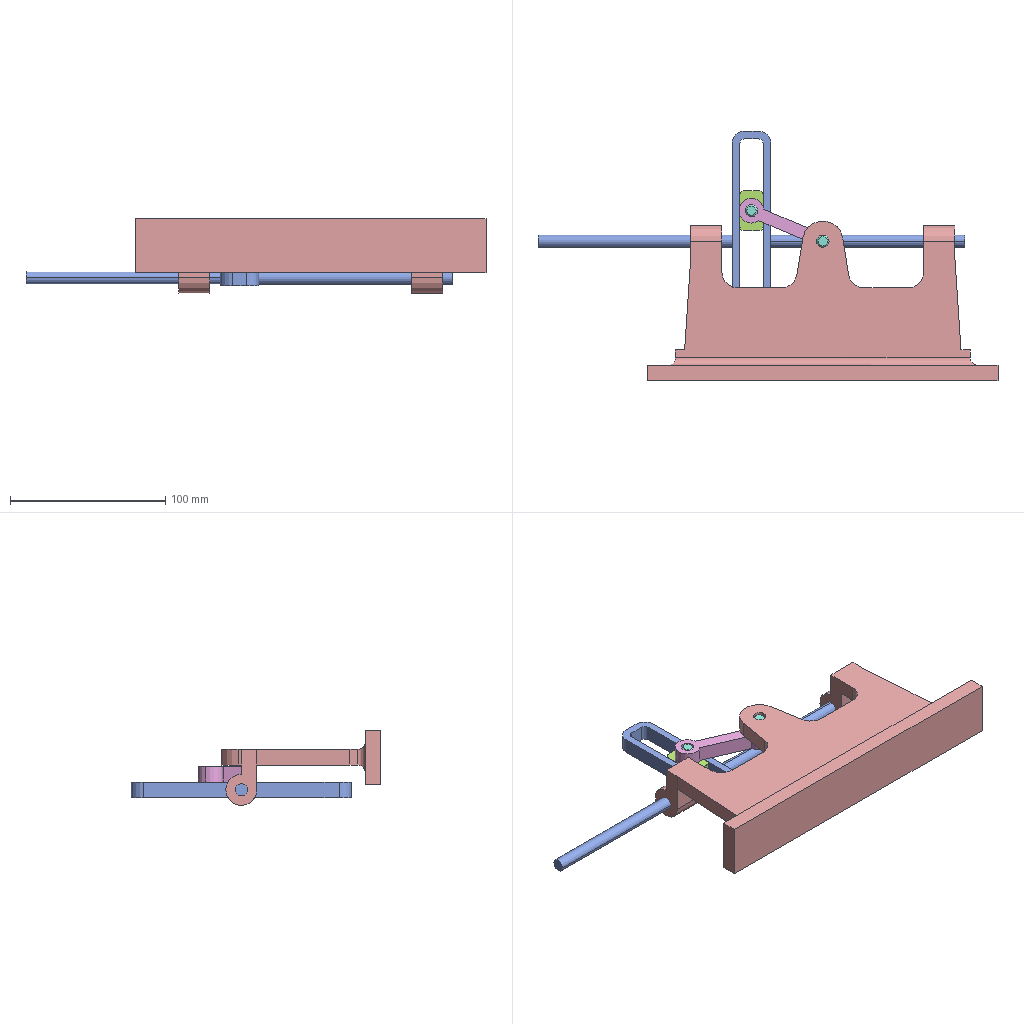Assembly | SolidWorks | 5 different items | 6 placed | box 296 x 161 x 48 mm
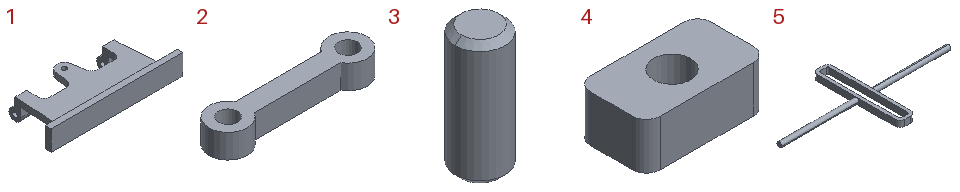Parts list (item | quantity | size | volume | features):
1 | x1 | 225.743 x 103 x 48.082 mm | 208388 mm3 | features ICE 2, Extrusion 1, Fillet 1, MirrorPattern 1
2 | x1 | 66 x 16 x 10 mm | 5791 mm3 | features Extrusion 1
3 | x2 | 8 x 8 x 20 mm | 982.271 mm3 | features Chamfer 1, Extrusion 1
4 | x1 | 26 x 15 x 10 mm | 3320 mm3 | features Extrusion 1, Fillet 1
5 | x1 | 275 x 142 x 10 mm | 27794 mm3 | features ICE 2, Extrusion 1
Mates (type | each side: item.copy, entity, surface, feature):
Concentric | 1.1 face cylinder Mirror1 | 5.1 face cylinder Boss-Extrude2
Parallel | 1.1 face plane Boss-Extrude1 | 5.1 face plane Boss-Extrude1
Coincident | 5.1 face plane Boss-Extrude1 | 4.1 face plane Boss-Extrude1 | 2 times
Concentric | 4.1 face cylinder Boss-Extrude1 | 2.1 face cylinder Boss-Extrude1
Concentric | 1.1 face cylinder Boss-Extrude1 | 2.1 face cylinder Boss-Extrude1
Coincident | 5.1 face plane Boss-Extrude1 | 2.1 face plane Boss-Extrude1
Concentric | 4.1 face cylinder Boss-Extrude1 | 3.1 face cylinder Boss-Extrude1
Coincident | 4.1 face plane Boss-Extrude1 | 3.1 face plane Boss-Extrude1
Concentric | 2.1 face cylinder Boss-Extrude1 | 3.2 face cylinder Boss-Extrude1
Coincident | 2.1 face plane Boss-Extrude1 | 3.2 face plane Boss-Extrude1